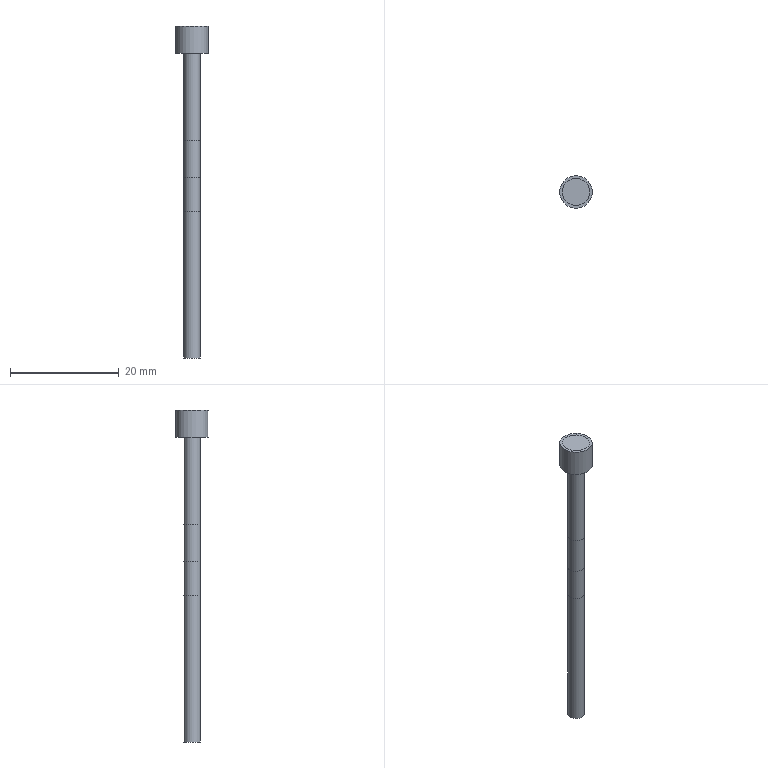Part | NX | features BREP 3 | 3 solids | 17 faces | box 6 x 6 x 61 mm | volume 951.587 mm3 | plane 9 | cylinder 7 | torus 1 | commonest cylinder face diameters 3 x3 2 x1 2.1 x1 5 x1 6 x1
STEP:
#1=CARTESIAN_POINT('',(2.5,0.,-5.));
#2=VERTEX_POINT('',#1);
#3=CARTESIAN_POINT('',(0.,0.,-5.));
#4=DIRECTION('',(0.,0.,-1.));
#5=DIRECTION('',(1.,0.,0.));
#6=AXIS2_PLACEMENT_3D('',#3,#4,#5);
#7=CIRCLE('',#6,2.5);
#8=EDGE_CURVE('',#2,#2,#7,.T.);
#9=ORIENTED_EDGE('',*,*,#8,.F.);
#10=EDGE_LOOP('',(#9));
#11=FACE_BOUND('',#10,.T.);
#12=CARTESIAN_POINT('',(2.5,0.,0.));
#13=VERTEX_POINT('',#12);
#14=CARTESIAN_POINT('',(0.,0.,0.));
#15=DIRECTION('',(0.,0.,-1.));
#16=DIRECTION('',(1.,0.,0.));
#17=AXIS2_PLACEMENT_3D('',#14,#15,#16);
#18=CIRCLE('',#17,2.5);
#19=EDGE_CURVE('',#13,#13,#18,.T.);
#20=ORIENTED_EDGE('',*,*,#19,.T.);
#21=EDGE_LOOP('',(#20));
#22=FACE_BOUND('',#21,.T.);
#23=CARTESIAN_POINT('',(0.,0.,-5.));
#24=DIRECTION('',(0.,0.,1.));
#25=DIRECTION('',(-1.,0.,0.));
#26=AXIS2_PLACEMENT_3D('',#23,#24,#25);
#27=CYLINDRICAL_SURFACE('',#26,2.5);
#28=ADVANCED_FACE('',(#11,#22),#27,.T.);
#29=CARTESIAN_POINT('',(-1.5,0.,-5.));
#30=VERTEX_POINT('',#29);
#31=CARTESIAN_POINT('',(0.,0.,-5.));
#32=DIRECTION('',(0.,0.,-1.));
#33=DIRECTION('',(-1.,0.,0.));
#34=AXIS2_PLACEMENT_3D('',#31,#32,#33);
#35=CIRCLE('',#34,1.5);
#36=EDGE_CURVE('',#30,#30,#35,.T.);
#37=ORIENTED_EDGE('',*,*,#36,.F.);
#38=EDGE_LOOP('',(#37));
#39=FACE_BOUND('',#38,.T.);
#40=ORIENTED_EDGE('',*,*,#8,.T.);
#41=EDGE_LOOP('',(#40));
#42=FACE_BOUND('',#41,.T.);
#43=CARTESIAN_POINT('',(0.,0.,-5.));
#44=DIRECTION('',(0.,0.,-1.));
#45=DIRECTION('',(1.,0.,0.));
#46=AXIS2_PLACEMENT_3D('',#43,#44,#45);
#47=PLANE('',#46);
#48=ADVANCED_FACE('',(#39,#42),#47,.T.);
#49=ORIENTED_EDGE('',*,*,#19,.F.);
#50=EDGE_LOOP('',(#49));
#51=FACE_BOUND('',#50,.T.);
#52=CARTESIAN_POINT('',(0.,0.,0.));
#53=DIRECTION('',(0.,0.,-1.));
#54=DIRECTION('',(1.,0.,0.));
#55=AXIS2_PLACEMENT_3D('',#52,#53,#54);
#56=PLANE('',#55);
#57=ADVANCED_FACE('',(#51),#56,.F.);
#58=ORIENTED_EDGE('',*,*,#36,.T.);
#59=EDGE_LOOP('',(#58));
#60=FACE_BOUND('',#59,.T.);
#61=CARTESIAN_POINT('',(-1.5,0.,-27.878));
#62=VERTEX_POINT('',#61);
#63=CARTESIAN_POINT('',(0.,0.,-27.878));
#64=DIRECTION('',(0.,0.,-1.));
#65=DIRECTION('',(-1.,0.,0.));
#66=AXIS2_PLACEMENT_3D('',#63,#64,#65);
#67=CIRCLE('',#66,1.5);
#68=EDGE_CURVE('',#62,#62,#67,.T.);
#69=ORIENTED_EDGE('',*,*,#68,.F.);
#70=EDGE_LOOP('',(#69));
#71=FACE_BOUND('',#70,.T.);
#72=CARTESIAN_POINT('',(0.,0.,-5.));
#73=DIRECTION('',(0.,0.,-1.));
#74=DIRECTION('',(1.,0.,0.));
#75=AXIS2_PLACEMENT_3D('',#72,#73,#74);
#76=CYLINDRICAL_SURFACE('',#75,1.5);
#77=ADVANCED_FACE('',(#60,#71),#76,.T.);
#78=ORIENTED_EDGE('',*,*,#68,.T.);
#79=EDGE_LOOP('',(#78));
#80=FACE_BOUND('',#79,.T.);
#81=CARTESIAN_POINT('',(-1.,0.,-31.));
#82=VERTEX_POINT('',#81);
#83=CARTESIAN_POINT('',(0.,0.,-31.));
#84=DIRECTION('',(0.,0.,-1.));
#85=DIRECTION('',(-1.,0.,0.));
#86=AXIS2_PLACEMENT_3D('',#83,#84,#85);
#87=CIRCLE('',#86,1.);
#88=EDGE_CURVE('',#82,#82,#87,.T.);
#89=ORIENTED_EDGE('',*,*,#88,.F.);
#90=EDGE_LOOP('',(#89));
#91=FACE_BOUND('',#90,.T.);
#92=CARTESIAN_POINT('',(0.,0.,-31.));
#93=DIRECTION('',(0.,0.,-1.));
#94=DIRECTION('',(1.,0.,0.));
#95=AXIS2_PLACEMENT_3D('',#92,#93,#94);
#96=TOROIDAL_SURFACE('',#95,11.,10.);
#97=ADVANCED_FACE('',(#80,#91),#96,.F.);
#98=ORIENTED_EDGE('',*,*,#88,.T.);
#99=EDGE_LOOP('',(#98));
#100=FACE_BOUND('',#99,.T.);
#101=CARTESIAN_POINT('',(1.,0.,-40.));
#102=VERTEX_POINT('',#101);
#103=CARTESIAN_POINT('',(0.,0.,-40.));
#104=DIRECTION('',(0.,0.,1.));
#105=DIRECTION('',(1.,0.,0.));
#106=AXIS2_PLACEMENT_3D('',#103,#104,#105);
#107=CIRCLE('',#106,1.);
#108=EDGE_CURVE('',#102,#102,#107,.T.);
#109=ORIENTED_EDGE('',*,*,#108,.T.);
#110=EDGE_LOOP('',(#109));
#111=FACE_BOUND('',#110,.T.);
#112=CARTESIAN_POINT('',(0.,0.,0.));
#113=DIRECTION('',(0.,0.,1.));
#114=DIRECTION('',(-1.,0.,0.));
#115=AXIS2_PLACEMENT_3D('',#112,#113,#114);
#116=CYLINDRICAL_SURFACE('',#115,1.);
#117=ADVANCED_FACE('',(#100,#111),#116,.T.);
#118=ORIENTED_EDGE('',*,*,#108,.F.);
#119=EDGE_LOOP('',(#118));
#120=FACE_BOUND('',#119,.T.);
#121=CARTESIAN_POINT('',(5.458,-13.172,-40.));
#122=DIRECTION('',(0.,0.,1.));
#123=DIRECTION('',(-1.,0.,0.));
#124=AXIS2_PLACEMENT_3D('',#121,#122,#123);
#125=PLANE('',#124);
#126=ADVANCED_FACE('',(#120),#125,.F.);
#127=CLOSED_SHELL('',(#28,#48,#57,#77,#97,#117,#126));
#128=MANIFOLD_SOLID_BREP('',#127);
#129=CARTESIAN_POINT('',(3.,0.,-5.));
#130=VERTEX_POINT('',#129);
#131=CARTESIAN_POINT('',(0.,0.,-5.));
#132=DIRECTION('',(0.,0.,-1.));
#133=DIRECTION('',(1.,0.,0.));
#134=AXIS2_PLACEMENT_3D('',#131,#132,#133);
#135=CIRCLE('',#134,3.);
#136=EDGE_CURVE('',#130,#130,#135,.T.);
#137=ORIENTED_EDGE('',*,*,#136,.F.);
#138=EDGE_LOOP('',(#137));
#139=FACE_BOUND('',#138,.T.);
#140=CARTESIAN_POINT('',(3.,0.,0.));
#141=VERTEX_POINT('',#140);
#142=CARTESIAN_POINT('',(0.,0.,0.));
#143=DIRECTION('',(0.,0.,-1.));
#144=DIRECTION('',(1.,0.,0.));
#145=AXIS2_PLACEMENT_3D('',#142,#143,#144);
#146=CIRCLE('',#145,3.);
#147=EDGE_CURVE('',#141,#141,#146,.T.);
#148=ORIENTED_EDGE('',*,*,#147,.T.);
#149=EDGE_LOOP('',(#148));
#150=FACE_BOUND('',#149,.T.);
#151=CARTESIAN_POINT('',(0.,0.,-5.));
#152=DIRECTION('',(0.,0.,1.));
#153=DIRECTION('',(-1.,0.,0.));
#154=AXIS2_PLACEMENT_3D('',#151,#152,#153);
#155=CYLINDRICAL_SURFACE('',#154,3.);
#156=ADVANCED_FACE('',(#139,#150),#155,.T.);
#157=CARTESIAN_POINT('',(-1.5,0.,-5.));
#158=VERTEX_POINT('',#157);
#159=CARTESIAN_POINT('',(0.,0.,-5.));
#160=DIRECTION('',(0.,0.,-1.));
#161=DIRECTION('',(-1.,0.,0.));
#162=AXIS2_PLACEMENT_3D('',#159,#160,#161);
#163=CIRCLE('',#162,1.5);
#164=EDGE_CURVE('',#158,#158,#163,.T.);
#165=ORIENTED_EDGE('',*,*,#164,.F.);
#166=EDGE_LOOP('',(#165));
#167=FACE_BOUND('',#166,.T.);
#168=ORIENTED_EDGE('',*,*,#136,.T.);
#169=EDGE_LOOP('',(#168));
#170=FACE_BOUND('',#169,.T.);
#171=CARTESIAN_POINT('',(0.,0.,-5.));
#172=DIRECTION('',(0.,0.,-1.));
#173=DIRECTION('',(1.,0.,0.));
#174=AXIS2_PLACEMENT_3D('',#171,#172,#173);
#175=PLANE('',#174);
#176=ADVANCED_FACE('',(#167,#170),#175,.T.);
#177=ORIENTED_EDGE('',*,*,#147,.F.);
#178=EDGE_LOOP('',(#177));
#179=FACE_BOUND('',#178,.T.);
#180=CARTESIAN_POINT('',(0.,0.,0.));
#181=DIRECTION('',(0.,0.,-1.));
#182=DIRECTION('',(1.,0.,0.));
#183=AXIS2_PLACEMENT_3D('',#180,#181,#182);
#184=PLANE('',#183);
#185=ADVANCED_FACE('',(#179),#184,.F.);
#186=CARTESIAN_POINT('',(1.05,0.,-34.));
#187=VERTEX_POINT('',#186);
#188=CARTESIAN_POINT('',(0.,0.,-34.));
#189=DIRECTION('',(0.,0.,1.));
#190=DIRECTION('',(1.,0.,0.));
#191=AXIS2_PLACEMENT_3D('',#188,#189,#190);
#192=CIRCLE('',#191,1.05);
#193=EDGE_CURVE('',#187,#187,#192,.T.);
#194=ORIENTED_EDGE('',*,*,#193,.T.);
#195=EDGE_LOOP('',(#194));
#196=FACE_BOUND('',#195,.T.);
#197=CARTESIAN_POINT('',(-1.5,0.,-34.));
#198=VERTEX_POINT('',#197);
#199=CARTESIAN_POINT('',(0.,0.,-34.));
#200=DIRECTION('',(0.,0.,-1.));
#201=DIRECTION('',(-1.,0.,0.));
#202=AXIS2_PLACEMENT_3D('',#199,#200,#201);
#203=CIRCLE('',#202,1.5);
#204=EDGE_CURVE('',#198,#198,#203,.T.);
#205=ORIENTED_EDGE('',*,*,#204,.T.);
#206=EDGE_LOOP('',(#205));
#207=FACE_BOUND('',#206,.T.);
#208=CARTESIAN_POINT('',(0.,0.,-34.));
#209=DIRECTION('',(0.,0.,-1.));
#210=DIRECTION('',(1.,0.,0.));
#211=AXIS2_PLACEMENT_3D('',#208,#209,#210);
#212=PLANE('',#211);
#213=ADVANCED_FACE('',(#196,#207),#212,.T.);
#214=ORIENTED_EDGE('',*,*,#204,.F.);
#215=EDGE_LOOP('',(#214));
#216=FACE_BOUND('',#215,.T.);
#217=ORIENTED_EDGE('',*,*,#164,.T.);
#218=EDGE_LOOP('',(#217));
#219=FACE_BOUND('',#218,.T.);
#220=CARTESIAN_POINT('',(0.,0.,-5.));
#221=DIRECTION('',(0.,0.,-1.));
#222=DIRECTION('',(1.,0.,0.));
#223=AXIS2_PLACEMENT_3D('',#220,#221,#222);
#224=CYLINDRICAL_SURFACE('',#223,1.5);
#225=ADVANCED_FACE('',(#216,#219),#224,.T.);
#226=CARTESIAN_POINT('',(1.05,0.,-40.));
#227=VERTEX_POINT('',#226);
#228=CARTESIAN_POINT('',(0.,0.,-40.));
#229=DIRECTION('',(0.,0.,1.));
#230=DIRECTION('',(1.,0.,0.));
#231=AXIS2_PLACEMENT_3D('',#228,#229,#230);
#232=CIRCLE('',#231,1.05);
#233=EDGE_CURVE('',#227,#227,#232,.T.);
#234=ORIENTED_EDGE('',*,*,#233,.T.);
#235=EDGE_LOOP('',(#234));
#236=FACE_BOUND('',#235,.T.);
#237=ORIENTED_EDGE('',*,*,#193,.F.);
#238=EDGE_LOOP('',(#237));
#239=FACE_BOUND('',#238,.T.);
#240=CARTESIAN_POINT('',(0.,0.,0.));
#241=DIRECTION('',(0.,0.,1.));
#242=DIRECTION('',(-1.,0.,0.));
#243=AXIS2_PLACEMENT_3D('',#240,#241,#242);
#244=CYLINDRICAL_SURFACE('',#243,1.05);
#245=ADVANCED_FACE('',(#236,#239),#244,.T.);
#246=ORIENTED_EDGE('',*,*,#233,.F.);
#247=EDGE_LOOP('',(#246));
#248=FACE_BOUND('',#247,.T.);
#249=CARTESIAN_POINT('',(5.458,-13.172,-40.));
#250=DIRECTION('',(0.,0.,1.));
#251=DIRECTION('',(-1.,0.,0.));
#252=AXIS2_PLACEMENT_3D('',#249,#250,#251);
#253=PLANE('',#252);
#254=ADVANCED_FACE('',(#248),#253,.F.);
#255=CLOSED_SHELL('',(#156,#176,#185,#213,#225,#245,#254));
#256=MANIFOLD_SOLID_BREP('',#255);
#257=CARTESIAN_POINT('',(-1.5,0.,-21.));
#258=VERTEX_POINT('',#257);
#259=CARTESIAN_POINT('',(0.,0.,-21.));
#260=DIRECTION('',(0.,0.,-1.));
#261=DIRECTION('',(-1.,0.,0.));
#262=AXIS2_PLACEMENT_3D('',#259,#260,#261);
#263=CIRCLE('',#262,1.5);
#264=EDGE_CURVE('',#258,#258,#263,.T.);
#265=ORIENTED_EDGE('',*,*,#264,.T.);
#266=EDGE_LOOP('',(#265));
#267=FACE_BOUND('',#266,.T.);
#268=CARTESIAN_POINT('',(-1.5,0.,-61.));
#269=VERTEX_POINT('',#268);
#270=CARTESIAN_POINT('',(0.,0.,-61.));
#271=DIRECTION('',(0.,0.,-1.));
#272=DIRECTION('',(-1.,0.,0.));
#273=AXIS2_PLACEMENT_3D('',#270,#271,#272);
#274=CIRCLE('',#273,1.5);
#275=EDGE_CURVE('',#269,#269,#274,.T.);
#276=ORIENTED_EDGE('',*,*,#275,.F.);
#277=EDGE_LOOP('',(#276));
#278=FACE_BOUND('',#277,.T.);
#279=CARTESIAN_POINT('',(0.,0.,-21.));
#280=DIRECTION('',(0.,0.,-1.));
#281=DIRECTION('',(1.,0.,0.));
#282=AXIS2_PLACEMENT_3D('',#279,#280,#281);
#283=CYLINDRICAL_SURFACE('',#282,1.5);
#284=ADVANCED_FACE('',(#267,#278),#283,.T.);
#285=ORIENTED_EDGE('',*,*,#264,.F.);
#286=EDGE_LOOP('',(#285));
#287=FACE_BOUND('',#286,.T.);
#288=CARTESIAN_POINT('',(0.,0.,-21.));
#289=DIRECTION('',(0.,0.,-1.));
#290=DIRECTION('',(1.,0.,0.));
#291=AXIS2_PLACEMENT_3D('',#288,#289,#290);
#292=PLANE('',#291);
#293=ADVANCED_FACE('',(#287),#292,.F.);
#294=ORIENTED_EDGE('',*,*,#275,.T.);
#295=EDGE_LOOP('',(#294));
#296=FACE_BOUND('',#295,.T.);
#297=CARTESIAN_POINT('',(0.,0.,-61.));
#298=DIRECTION('',(0.,0.,-1.));
#299=DIRECTION('',(1.,0.,0.));
#300=AXIS2_PLACEMENT_3D('',#297,#298,#299);
#301=PLANE('',#300);
#302=ADVANCED_FACE('',(#296),#301,.T.);
#303=CLOSED_SHELL('',(#284,#293,#302));
#304=MANIFOLD_SOLID_BREP('',#303);
#305=(LENGTH_UNIT()NAMED_UNIT(*)SI_UNIT(.MILLI.,.METRE.));
#306=UNCERTAINTY_MEASURE_WITH_UNIT(LENGTH_MEASURE(0.00001),#305,'','');
#307=(NAMED_UNIT(*)PLANE_ANGLE_UNIT()SI_UNIT($,.RADIAN.));
#308=(NAMED_UNIT(*)SI_UNIT($,.STERADIAN.)SOLID_ANGLE_UNIT());
#309=(GEOMETRIC_REPRESENTATION_CONTEXT(3)GLOBAL_UNCERTAINTY_ASSIGNED_CONTEXT((#306))GLOBAL_UNIT_ASSIGNED_CONTEXT((#305,#307,#308))REPRESENTATION_CONTEXT('',''));
#310=ADVANCED_BREP_SHAPE_REPRESENTATION('',(#128,#256,#304),#309);